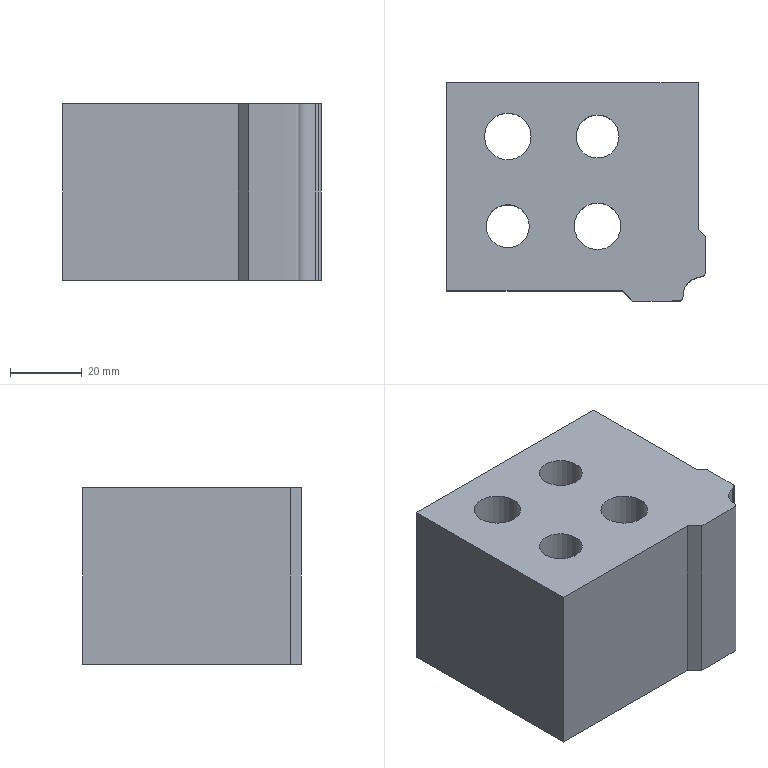Part | NX | features solid 2 | 1 solid | 20 faces | box 72 x 60.859 x 49.284 mm | volume 170289 mm3 | plane 11 | cylinder 7 | spline 2 | commonest cylinder face diameters 12 x2 13 x2 20 x2 2 x1
STEP:
#1=CARTESIAN_POINT('',(-548.,845.,-149.284));
#2=VERTEX_POINT('',#1);
#3=CARTESIAN_POINT('',(-538.,845.,-149.284));
#4=DIRECTION('',(0.,0.,-1.));
#5=DIRECTION('',(-1.,0.,0.));
#6=AXIS2_PLACEMENT_3D('',#3,#4,#5);
#7=CIRCLE('',#6,10.);
#8=EDGE_CURVE('',#2,#2,#7,.T.);
#9=ORIENTED_EDGE('',*,*,#8,.F.);
#10=EDGE_LOOP('',(#9));
#11=FACE_BOUND('',#10,.T.);
#12=CARTESIAN_POINT('',(-544.,820.,-149.284));
#13=VERTEX_POINT('',#12);
#14=CARTESIAN_POINT('',(-538.,820.,-149.284));
#15=DIRECTION('',(0.,0.,-1.));
#16=DIRECTION('',(-1.,0.,0.));
#17=AXIS2_PLACEMENT_3D('',#14,#15,#16);
#18=CIRCLE('',#17,6.);
#19=EDGE_CURVE('',#13,#13,#18,.T.);
#20=ORIENTED_EDGE('',*,*,#19,.F.);
#21=EDGE_LOOP('',(#20));
#22=FACE_BOUND('',#21,.T.);
#23=CARTESIAN_POINT('',(-519.,845.,-149.284));
#24=VERTEX_POINT('',#23);
#25=CARTESIAN_POINT('',(-513.,845.,-149.284));
#26=DIRECTION('',(0.,0.,-1.));
#27=DIRECTION('',(-1.,0.,0.));
#28=AXIS2_PLACEMENT_3D('',#25,#26,#27);
#29=CIRCLE('',#28,6.);
#30=EDGE_CURVE('',#24,#24,#29,.T.);
#31=ORIENTED_EDGE('',*,*,#30,.F.);
#32=EDGE_LOOP('',(#31));
#33=FACE_BOUND('',#32,.T.);
#34=CARTESIAN_POINT('',(-523.,820.,-149.284));
#35=VERTEX_POINT('',#34);
#36=CARTESIAN_POINT('',(-513.,820.,-149.284));
#37=DIRECTION('',(0.,0.,-1.));
#38=DIRECTION('',(-1.,0.,0.));
#39=AXIS2_PLACEMENT_3D('',#36,#37,#38);
#40=CIRCLE('',#39,10.);
#41=EDGE_CURVE('',#35,#35,#40,.T.);
#42=ORIENTED_EDGE('',*,*,#41,.F.);
#43=EDGE_LOOP('',(#42));
#44=FACE_BOUND('',#43,.T.);
#45=CARTESIAN_POINT('',(-503.223,799.156,-149.284));
#46=VERTEX_POINT('',#45);
#47=CARTESIAN_POINT('',(-484.629,805.851,-149.284));
#48=VERTEX_POINT('',#47);
#49=CARTESIAN_POINT('',(-534.002,799.156,-149.284));
#50=CARTESIAN_POINT('',(-520.407,799.156,-149.284));
#51=CARTESIAN_POINT('',(-506.812,799.156,-149.284));
#52=CARTESIAN_POINT('',(-493.216,799.156,-149.284));
#53=CARTESIAN_POINT('',(-492.716,799.156,-149.284));
#54=CARTESIAN_POINT('',(-491.716,799.156,-149.284));
#55=CARTESIAN_POINT('',(-490.649,799.128,-149.284));
#56=CARTESIAN_POINT('',(-490.021,799.17,-149.284));
#57=CARTESIAN_POINT('',(-489.772,799.252,-149.284));
#58=CARTESIAN_POINT('',(-489.501,799.442,-149.284));
#59=CARTESIAN_POINT('',(-489.316,799.721,-149.284));
#60=CARTESIAN_POINT('',(-489.236,799.97,-149.284));
#61=CARTESIAN_POINT('',(-489.184,800.499,-149.284));
#62=CARTESIAN_POINT('',(-489.152,801.357,-149.284));
#63=CARTESIAN_POINT('',(-488.826,802.918,-149.284));
#64=CARTESIAN_POINT('',(-487.668,804.644,-149.284));
#65=CARTESIAN_POINT('',(-485.756,805.629,-149.284));
#66=CARTESIAN_POINT('',(-484.079,805.973,-149.284));
#67=CARTESIAN_POINT('',(-483.087,806.009,-149.284));
#68=CARTESIAN_POINT('',(-482.401,806.124,-149.284));
#69=CARTESIAN_POINT('',(-482.07,806.341,-149.284));
#70=CARTESIAN_POINT('',(-481.846,806.67,-149.284));
#71=CARTESIAN_POINT('',(-481.753,807.261,-149.284));
#72=CARTESIAN_POINT('',(-481.79,808.059,-149.284));
#73=CARTESIAN_POINT('',(-481.79,808.726,-149.284));
#74=CARTESIAN_POINT('',(-481.79,809.059,-149.284));
#75=CARTESIAN_POINT('',(-481.79,822.654,-149.284));
#76=CARTESIAN_POINT('',(-481.79,836.249,-149.284));
#77=CARTESIAN_POINT('',(-481.79,849.844,-149.284));
#78=B_SPLINE_CURVE_WITH_KNOTS('',3,(#49,#50,#51,#52,#53,#54,#55,#56,#57,#58,#59,#60,#61,#62,#63,#64,#65,#66,#67,#68,#69,#70,#71,#72,#73,#74,#75,#76,#77),.UNSPECIFIED.,.F.,.F.,(4,3,1,1,1,1,1,1,1,1,1,1,1,1,1,1,1,1,1,1,1,3,4),(0.,0.4079,0.4228,0.4378,0.4398,0.4418,0.4457,0.4496,0.4516,0.4536,0.4664,0.4793,0.5051,0.5308,0.5437,0.5566,0.5605,0.5644,0.5683,0.5722,0.5822,0.5921,1.),.UNSPECIFIED.);
#79=EDGE_CURVE('',#46,#48,#78,.T.);
#80=ORIENTED_EDGE('',*,*,#79,.F.);
#81=CARTESIAN_POINT('',(-506.067,802.,-149.284));
#82=VERTEX_POINT('',#81);
#83=CARTESIAN_POINT('',(-499.067,795.,-149.284));
#84=DIRECTION('',(-0.7071,0.7071,0.));
#85=VECTOR('',#84,1000.);
#86=LINE('',#83,#85);
#87=EDGE_CURVE('',#82,#46,#86,.F.);
#88=ORIENTED_EDGE('',*,*,#87,.F.);
#89=CARTESIAN_POINT('',(-555.,802.,-149.284));
#90=VERTEX_POINT('',#89);
#91=CARTESIAN_POINT('',(-504.067,802.,-149.284));
#92=DIRECTION('',(-1.,0.,0.));
#93=VECTOR('',#92,1000.);
#94=LINE('',#91,#93);
#95=EDGE_CURVE('',#90,#82,#94,.F.);
#96=ORIENTED_EDGE('',*,*,#95,.F.);
#97=CARTESIAN_POINT('',(-555.,860.,-149.284));
#98=VERTEX_POINT('',#97);
#99=CARTESIAN_POINT('',(-555.,800.,-149.284));
#100=DIRECTION('',(0.,1.,0.));
#101=VECTOR('',#100,1000.);
#102=LINE('',#99,#101);
#103=EDGE_CURVE('',#98,#90,#102,.F.);
#104=ORIENTED_EDGE('',*,*,#103,.F.);
#105=CARTESIAN_POINT('',(-485.,860.,-149.284));
#106=VERTEX_POINT('',#105);
#107=CARTESIAN_POINT('',(-488.,860.,-149.284));
#108=DIRECTION('',(-1.,0.,0.));
#109=VECTOR('',#108,1000.);
#110=LINE('',#107,#109);
#111=EDGE_CURVE('',#98,#106,#110,.F.);
#112=ORIENTED_EDGE('',*,*,#111,.T.);
#113=CARTESIAN_POINT('',(-485.,819.091,-149.284));
#114=VERTEX_POINT('',#113);
#115=CARTESIAN_POINT('',(-485.,822.091,-149.284));
#116=DIRECTION('',(0.,1.,0.));
#117=VECTOR('',#116,1000.);
#118=LINE('',#115,#117);
#119=EDGE_CURVE('',#106,#114,#118,.F.);
#120=ORIENTED_EDGE('',*,*,#119,.T.);
#121=CARTESIAN_POINT('',(-483.,817.091,-149.284));
#122=VERTEX_POINT('',#121);
#123=CARTESIAN_POINT('',(-483.,817.091,-149.284));
#124=DIRECTION('',(-0.7071,0.7071,0.));
#125=VECTOR('',#124,1000.);
#126=LINE('',#123,#125);
#127=EDGE_CURVE('',#114,#122,#126,.F.);
#128=ORIENTED_EDGE('',*,*,#127,.T.);
#129=CARTESIAN_POINT('',(-483.,807.091,-149.284));
#130=VERTEX_POINT('',#129);
#131=CARTESIAN_POINT('',(-483.,807.091,-149.284));
#132=DIRECTION('',(0.,1.,0.));
#133=VECTOR('',#132,1000.);
#134=LINE('',#131,#133);
#135=EDGE_CURVE('',#122,#130,#134,.F.);
#136=ORIENTED_EDGE('',*,*,#135,.T.);
#137=CARTESIAN_POINT('',(-483.777,806.116,-149.284));
#138=VERTEX_POINT('',#137);
#139=CARTESIAN_POINT('',(-484.,807.091,-149.284));
#140=DIRECTION('',(0.,0.,-1.));
#141=DIRECTION('',(-1.,0.,0.));
#142=AXIS2_PLACEMENT_3D('',#139,#140,#141);
#143=CIRCLE('',#142,1.);
#144=EDGE_CURVE('',#130,#138,#143,.T.);
#145=ORIENTED_EDGE('',*,*,#144,.T.);
#146=CARTESIAN_POINT('',(-483.777,806.116,-149.284));
#147=CARTESIAN_POINT('',(-484.07,806.049,-149.284));
#148=CARTESIAN_POINT('',(-484.354,805.962,-149.284));
#149=CARTESIAN_POINT('',(-484.629,805.851,-149.284));
#150=B_SPLINE_CURVE_WITH_KNOTS('',3,(#146,#147,#148,#149),.UNSPECIFIED.,.F.,.F.,(4,4),(0.,0.000889),.UNSPECIFIED.);
#151=EDGE_CURVE('',#138,#48,#150,.T.);
#152=ORIENTED_EDGE('',*,*,#151,.T.);
#153=EDGE_LOOP('',(#80,#88,#96,#104,#112,#120,#128,#136,#145,#152));
#154=FACE_BOUND('',#153,.T.);
#155=CARTESIAN_POINT('',(-594.308,845.,-149.284));
#156=DIRECTION('',(0.,0.,-1.));
#157=DIRECTION('',(-1.,0.,0.));
#158=AXIS2_PLACEMENT_3D('',#155,#156,#157);
#159=PLANE('',#158);
#160=ADVANCED_FACE('',(#11,#22,#33,#44,#154),#159,.T.);
#161=CARTESIAN_POINT('',(-484.629,805.851,-100.));
#162=VERTEX_POINT('',#161);
#163=CARTESIAN_POINT('',(-503.223,799.156,-100.));
#164=VERTEX_POINT('',#163);
#165=CARTESIAN_POINT('',(-534.002,799.156,-100.));
#166=CARTESIAN_POINT('',(-520.407,799.156,-100.));
#167=CARTESIAN_POINT('',(-506.812,799.156,-100.));
#168=CARTESIAN_POINT('',(-493.216,799.156,-100.));
#169=CARTESIAN_POINT('',(-492.716,799.156,-100.));
#170=CARTESIAN_POINT('',(-491.716,799.156,-100.));
#171=CARTESIAN_POINT('',(-490.649,799.128,-100.));
#172=CARTESIAN_POINT('',(-490.021,799.17,-100.));
#173=CARTESIAN_POINT('',(-489.772,799.252,-100.));
#174=CARTESIAN_POINT('',(-489.501,799.442,-100.));
#175=CARTESIAN_POINT('',(-489.316,799.721,-100.));
#176=CARTESIAN_POINT('',(-489.236,799.97,-100.));
#177=CARTESIAN_POINT('',(-489.184,800.499,-100.));
#178=CARTESIAN_POINT('',(-489.152,801.357,-100.));
#179=CARTESIAN_POINT('',(-488.826,802.918,-100.));
#180=CARTESIAN_POINT('',(-487.668,804.644,-100.));
#181=CARTESIAN_POINT('',(-485.756,805.629,-100.));
#182=CARTESIAN_POINT('',(-484.079,805.973,-100.));
#183=CARTESIAN_POINT('',(-483.087,806.009,-100.));
#184=CARTESIAN_POINT('',(-482.401,806.124,-100.));
#185=CARTESIAN_POINT('',(-482.07,806.341,-100.));
#186=CARTESIAN_POINT('',(-481.846,806.67,-100.));
#187=CARTESIAN_POINT('',(-481.753,807.261,-100.));
#188=CARTESIAN_POINT('',(-481.79,808.059,-100.));
#189=CARTESIAN_POINT('',(-481.79,808.726,-100.));
#190=CARTESIAN_POINT('',(-481.79,809.059,-100.));
#191=CARTESIAN_POINT('',(-481.79,822.654,-100.));
#192=CARTESIAN_POINT('',(-481.79,836.249,-100.));
#193=CARTESIAN_POINT('',(-481.79,849.844,-100.));
#194=B_SPLINE_CURVE_WITH_KNOTS('',3,(#165,#166,#167,#168,#169,#170,#171,#172,#173,#174,#175,#176,#177,#178,#179,#180,#181,#182,#183,#184,#185,#186,#187,#188,#189,#190,#191,#192,#193),.UNSPECIFIED.,.F.,.F.,(4,3,1,1,1,1,1,1,1,1,1,1,1,1,1,1,1,1,1,1,1,3,4),(0.,0.4079,0.4228,0.4378,0.4398,0.4418,0.4457,0.4496,0.4516,0.4536,0.4664,0.4793,0.5051,0.5308,0.5437,0.5566,0.5605,0.5644,0.5683,0.5722,0.5822,0.5921,1.),.UNSPECIFIED.);
#195=EDGE_CURVE('',#162,#164,#194,.F.);
#196=ORIENTED_EDGE('',*,*,#195,.F.);
#197=CARTESIAN_POINT('',(-483.777,806.116,-100.));
#198=VERTEX_POINT('',#197);
#199=CARTESIAN_POINT('',(-484.629,805.851,-100.));
#200=CARTESIAN_POINT('',(-484.353,805.962,-100.));
#201=CARTESIAN_POINT('',(-484.069,806.049,-100.));
#202=CARTESIAN_POINT('',(-483.777,806.116,-100.));
#203=B_SPLINE_CURVE_WITH_KNOTS('',3,(#199,#200,#201,#202),.UNSPECIFIED.,.F.,.F.,(4,4),(0.06032,0.06122),.UNSPECIFIED.);
#204=EDGE_CURVE('',#162,#198,#203,.T.);
#205=ORIENTED_EDGE('',*,*,#204,.T.);
#206=CARTESIAN_POINT('',(-483.,807.091,-100.));
#207=VERTEX_POINT('',#206);
#208=CARTESIAN_POINT('',(-484.,807.091,-100.));
#209=DIRECTION('',(0.,0.,1.));
#210=DIRECTION('',(1.,0.,0.));
#211=AXIS2_PLACEMENT_3D('',#208,#209,#210);
#212=CIRCLE('',#211,1.);
#213=EDGE_CURVE('',#198,#207,#212,.T.);
#214=ORIENTED_EDGE('',*,*,#213,.T.);
#215=CARTESIAN_POINT('',(-483.,817.091,-100.));
#216=VERTEX_POINT('',#215);
#217=CARTESIAN_POINT('',(-483.,808.547,-100.));
#218=DIRECTION('',(0.,1.,0.));
#219=VECTOR('',#218,1000.);
#220=LINE('',#217,#219);
#221=EDGE_CURVE('',#207,#216,#220,.T.);
#222=ORIENTED_EDGE('',*,*,#221,.T.);
#223=CARTESIAN_POINT('',(-485.,819.091,-100.));
#224=VERTEX_POINT('',#223);
#225=CARTESIAN_POINT('',(-485.119,819.209,-100.));
#226=DIRECTION('',(-0.7071,0.7071,0.));
#227=VECTOR('',#226,1000.);
#228=LINE('',#225,#227);
#229=EDGE_CURVE('',#216,#224,#228,.T.);
#230=ORIENTED_EDGE('',*,*,#229,.T.);
#231=CARTESIAN_POINT('',(-485.,860.,-100.));
#232=VERTEX_POINT('',#231);
#233=CARTESIAN_POINT('',(-485.,808.547,-100.));
#234=DIRECTION('',(0.,1.,0.));
#235=VECTOR('',#234,1000.);
#236=LINE('',#233,#235);
#237=EDGE_CURVE('',#224,#232,#236,.T.);
#238=ORIENTED_EDGE('',*,*,#237,.T.);
#239=CARTESIAN_POINT('',(-555.,860.,-100.));
#240=VERTEX_POINT('',#239);
#241=CARTESIAN_POINT('',(-495.781,860.,-100.));
#242=DIRECTION('',(-1.,0.,0.));
#243=VECTOR('',#242,1000.);
#244=LINE('',#241,#243);
#245=EDGE_CURVE('',#232,#240,#244,.T.);
#246=ORIENTED_EDGE('',*,*,#245,.T.);
#247=CARTESIAN_POINT('',(-555.,802.,-100.));
#248=VERTEX_POINT('',#247);
#249=CARTESIAN_POINT('',(-555.,808.547,-100.));
#250=DIRECTION('',(0.,1.,0.));
#251=VECTOR('',#250,1000.);
#252=LINE('',#249,#251);
#253=EDGE_CURVE('',#248,#240,#252,.T.);
#254=ORIENTED_EDGE('',*,*,#253,.F.);
#255=CARTESIAN_POINT('',(-506.067,802.,-100.));
#256=VERTEX_POINT('',#255);
#257=CARTESIAN_POINT('',(-495.781,802.,-100.));
#258=DIRECTION('',(-1.,0.,0.));
#259=VECTOR('',#258,1000.);
#260=LINE('',#257,#259);
#261=EDGE_CURVE('',#256,#248,#260,.T.);
#262=ORIENTED_EDGE('',*,*,#261,.F.);
#263=CARTESIAN_POINT('',(-504.197,800.131,-100.));
#264=DIRECTION('',(-0.7071,0.7071,0.));
#265=VECTOR('',#264,1000.);
#266=LINE('',#263,#265);
#267=EDGE_CURVE('',#164,#256,#266,.T.);
#268=ORIENTED_EDGE('',*,*,#267,.F.);
#269=EDGE_LOOP('',(#196,#205,#214,#222,#230,#238,#246,#254,#262,#268));
#270=FACE_BOUND('',#269,.T.);
#271=CARTESIAN_POINT('',(-506.5,820.,-100.));
#272=VERTEX_POINT('',#271);
#273=CARTESIAN_POINT('',(-513.,820.,-100.));
#274=DIRECTION('',(0.,0.,1.));
#275=DIRECTION('',(1.,0.,0.));
#276=AXIS2_PLACEMENT_3D('',#273,#274,#275);
#277=CIRCLE('',#276,6.5);
#278=EDGE_CURVE('',#272,#272,#277,.T.);
#279=ORIENTED_EDGE('',*,*,#278,.F.);
#280=EDGE_LOOP('',(#279));
#281=FACE_BOUND('',#280,.T.);
#282=CARTESIAN_POINT('',(-531.5,845.,-100.));
#283=VERTEX_POINT('',#282);
#284=CARTESIAN_POINT('',(-538.,845.,-100.));
#285=DIRECTION('',(0.,0.,1.));
#286=DIRECTION('',(1.,0.,0.));
#287=AXIS2_PLACEMENT_3D('',#284,#285,#286);
#288=CIRCLE('',#287,6.5);
#289=EDGE_CURVE('',#283,#283,#288,.T.);
#290=ORIENTED_EDGE('',*,*,#289,.F.);
#291=EDGE_LOOP('',(#290));
#292=FACE_BOUND('',#291,.T.);
#293=CARTESIAN_POINT('',(-507.,845.,-100.));
#294=VERTEX_POINT('',#293);
#295=CARTESIAN_POINT('',(-513.,845.,-100.));
#296=DIRECTION('',(0.,0.,1.));
#297=DIRECTION('',(1.,0.,0.));
#298=AXIS2_PLACEMENT_3D('',#295,#296,#297);
#299=CIRCLE('',#298,6.);
#300=EDGE_CURVE('',#294,#294,#299,.F.);
#301=ORIENTED_EDGE('',*,*,#300,.T.);
#302=EDGE_LOOP('',(#301));
#303=FACE_BOUND('',#302,.T.);
#304=CARTESIAN_POINT('',(-532.,820.,-100.));
#305=VERTEX_POINT('',#304);
#306=CARTESIAN_POINT('',(-538.,820.,-100.));
#307=DIRECTION('',(0.,0.,1.));
#308=DIRECTION('',(1.,0.,0.));
#309=AXIS2_PLACEMENT_3D('',#306,#307,#308);
#310=CIRCLE('',#309,6.);
#311=EDGE_CURVE('',#305,#305,#310,.F.);
#312=ORIENTED_EDGE('',*,*,#311,.T.);
#313=EDGE_LOOP('',(#312));
#314=FACE_BOUND('',#313,.T.);
#315=CARTESIAN_POINT('',(-495.781,808.547,-100.));
#316=DIRECTION('',(0.,0.,1.));
#317=DIRECTION('',(1.,0.,0.));
#318=AXIS2_PLACEMENT_3D('',#315,#316,#317);
#319=PLANE('',#318);
#320=ADVANCED_FACE('',(#270,#281,#292,#303,#314),#319,.T.);
#321=CARTESIAN_POINT('',(-555.,860.,-505.));
#322=DIRECTION('',(0.,0.,1.));
#323=VECTOR('',#322,1000.);
#324=LINE('',#321,#323);
#325=EDGE_CURVE('',#98,#240,#324,.T.);
#326=ORIENTED_EDGE('',*,*,#325,.F.);
#327=ORIENTED_EDGE('',*,*,#103,.T.);
#328=CARTESIAN_POINT('',(-555.,802.,-505.));
#329=DIRECTION('',(0.,0.,1.));
#330=VECTOR('',#329,1000.);
#331=LINE('',#328,#330);
#332=EDGE_CURVE('',#90,#248,#331,.T.);
#333=ORIENTED_EDGE('',*,*,#332,.T.);
#334=ORIENTED_EDGE('',*,*,#253,.T.);
#335=EDGE_LOOP('',(#326,#327,#333,#334));
#336=FACE_BOUND('',#335,.T.);
#337=CARTESIAN_POINT('',(-555.,800.,-505.));
#338=DIRECTION('',(1.,0.,0.));
#339=DIRECTION('',(0.,0.,-1.));
#340=AXIS2_PLACEMENT_3D('',#337,#338,#339);
#341=PLANE('',#340);
#342=ADVANCED_FACE('',(#336),#341,.F.);
#343=ORIENTED_EDGE('',*,*,#332,.F.);
#344=ORIENTED_EDGE('',*,*,#95,.T.);
#345=CARTESIAN_POINT('',(-506.067,802.,-505.));
#346=DIRECTION('',(0.,0.,1.));
#347=VECTOR('',#346,1000.);
#348=LINE('',#345,#347);
#349=EDGE_CURVE('',#82,#256,#348,.T.);
#350=ORIENTED_EDGE('',*,*,#349,.T.);
#351=ORIENTED_EDGE('',*,*,#261,.T.);
#352=EDGE_LOOP('',(#343,#344,#350,#351));
#353=FACE_BOUND('',#352,.T.);
#354=CARTESIAN_POINT('',(-504.067,802.,-505.));
#355=DIRECTION('',(0.,1.,0.));
#356=DIRECTION('',(0.,0.,1.));
#357=AXIS2_PLACEMENT_3D('',#354,#355,#356);
#358=PLANE('',#357);
#359=ADVANCED_FACE('',(#353),#358,.F.);
#360=ORIENTED_EDGE('',*,*,#87,.T.);
#361=CARTESIAN_POINT('',(-503.223,799.156,495.));
#362=DIRECTION('',(0.,0.,-1.));
#363=VECTOR('',#362,1000.);
#364=LINE('',#361,#363);
#365=EDGE_CURVE('',#46,#164,#364,.F.);
#366=ORIENTED_EDGE('',*,*,#365,.T.);
#367=ORIENTED_EDGE('',*,*,#267,.T.);
#368=ORIENTED_EDGE('',*,*,#349,.F.);
#369=EDGE_LOOP('',(#360,#366,#367,#368));
#370=FACE_BOUND('',#369,.T.);
#371=CARTESIAN_POINT('',(-499.067,795.,-505.));
#372=DIRECTION('',(0.7071,0.7071,0.));
#373=DIRECTION('',(-0.7071,0.7071,0.));
#374=AXIS2_PLACEMENT_3D('',#371,#372,#373);
#375=PLANE('',#374);
#376=ADVANCED_FACE('',(#370),#375,.F.);
#377=CARTESIAN_POINT('',(-484.629,805.851,495.));
#378=DIRECTION('',(0.,0.,-1.));
#379=VECTOR('',#378,1000.);
#380=LINE('',#377,#379);
#381=EDGE_CURVE('',#48,#162,#380,.F.);
#382=ORIENTED_EDGE('',*,*,#381,.F.);
#383=ORIENTED_EDGE('',*,*,#151,.F.);
#384=CARTESIAN_POINT('',(-483.777,806.116,-505.));
#385=DIRECTION('',(0.,0.,1.));
#386=VECTOR('',#385,1000.);
#387=LINE('',#384,#386);
#388=EDGE_CURVE('',#138,#198,#387,.T.);
#389=ORIENTED_EDGE('',*,*,#388,.T.);
#390=ORIENTED_EDGE('',*,*,#204,.F.);
#391=EDGE_LOOP('',(#382,#383,#389,#390));
#392=FACE_BOUND('',#391,.T.);
#393=CARTESIAN_POINT('',(-484.629,805.851,-149.284));
#394=CARTESIAN_POINT('',(-484.629,805.851,-100.));
#395=CARTESIAN_POINT('',(-484.354,805.962,-149.284));
#396=CARTESIAN_POINT('',(-484.354,805.962,-100.));
#397=CARTESIAN_POINT('',(-484.069,806.049,-149.284));
#398=CARTESIAN_POINT('',(-484.069,806.049,-100.));
#399=CARTESIAN_POINT('',(-483.777,806.116,-149.284));
#400=CARTESIAN_POINT('',(-483.777,806.116,-100.));
#401=B_SPLINE_SURFACE_WITH_KNOTS('',3,1,((#393,#394),(#395,#396),(#397,#398),(#399,#400)),.SURF_OF_LINEAR_EXTRUSION.,.F.,.F.,.F.,(4,4),(2,2),(0.9197,0.987),(0.,1.),.PIECEWISE_BEZIER_KNOTS.);
#402=ADVANCED_FACE('',(#392),#401,.T.);
#403=ORIENTED_EDGE('',*,*,#144,.F.);
#404=CARTESIAN_POINT('',(-483.,807.091,-505.));
#405=DIRECTION('',(0.,0.,1.));
#406=VECTOR('',#405,1000.);
#407=LINE('',#404,#406);
#408=EDGE_CURVE('',#130,#207,#407,.T.);
#409=ORIENTED_EDGE('',*,*,#408,.T.);
#410=ORIENTED_EDGE('',*,*,#213,.F.);
#411=ORIENTED_EDGE('',*,*,#388,.F.);
#412=EDGE_LOOP('',(#403,#409,#410,#411));
#413=FACE_BOUND('',#412,.T.);
#414=CARTESIAN_POINT('',(-484.,807.091,-505.));
#415=DIRECTION('',(0.,0.,1.));
#416=DIRECTION('',(1.,0.,0.));
#417=AXIS2_PLACEMENT_3D('',#414,#415,#416);
#418=CYLINDRICAL_SURFACE('',#417,1.);
#419=ADVANCED_FACE('',(#413),#418,.T.);
#420=ORIENTED_EDGE('',*,*,#135,.F.);
#421=CARTESIAN_POINT('',(-483.,817.091,-505.));
#422=DIRECTION('',(0.,0.,1.));
#423=VECTOR('',#422,1000.);
#424=LINE('',#421,#423);
#425=EDGE_CURVE('',#122,#216,#424,.T.);
#426=ORIENTED_EDGE('',*,*,#425,.T.);
#427=ORIENTED_EDGE('',*,*,#221,.F.);
#428=ORIENTED_EDGE('',*,*,#408,.F.);
#429=EDGE_LOOP('',(#420,#426,#427,#428));
#430=FACE_BOUND('',#429,.T.);
#431=CARTESIAN_POINT('',(-483.,807.091,-505.));
#432=DIRECTION('',(1.,0.,0.));
#433=DIRECTION('',(0.,0.,-1.));
#434=AXIS2_PLACEMENT_3D('',#431,#432,#433);
#435=PLANE('',#434);
#436=ADVANCED_FACE('',(#430),#435,.T.);
#437=ORIENTED_EDGE('',*,*,#127,.F.);
#438=CARTESIAN_POINT('',(-485.,819.091,-505.));
#439=DIRECTION('',(0.,0.,1.));
#440=VECTOR('',#439,1000.);
#441=LINE('',#438,#440);
#442=EDGE_CURVE('',#114,#224,#441,.T.);
#443=ORIENTED_EDGE('',*,*,#442,.T.);
#444=ORIENTED_EDGE('',*,*,#229,.F.);
#445=ORIENTED_EDGE('',*,*,#425,.F.);
#446=EDGE_LOOP('',(#437,#443,#444,#445));
#447=FACE_BOUND('',#446,.T.);
#448=CARTESIAN_POINT('',(-483.,817.091,-505.));
#449=DIRECTION('',(0.7071,0.7071,0.));
#450=DIRECTION('',(-0.7071,0.7071,0.));
#451=AXIS2_PLACEMENT_3D('',#448,#449,#450);
#452=PLANE('',#451);
#453=ADVANCED_FACE('',(#447),#452,.T.);
#454=ORIENTED_EDGE('',*,*,#119,.F.);
#455=CARTESIAN_POINT('',(-485.,860.,-505.));
#456=DIRECTION('',(0.,0.,1.));
#457=VECTOR('',#456,1000.);
#458=LINE('',#455,#457);
#459=EDGE_CURVE('',#106,#232,#458,.T.);
#460=ORIENTED_EDGE('',*,*,#459,.T.);
#461=ORIENTED_EDGE('',*,*,#237,.F.);
#462=ORIENTED_EDGE('',*,*,#442,.F.);
#463=EDGE_LOOP('',(#454,#460,#461,#462));
#464=FACE_BOUND('',#463,.T.);
#465=CARTESIAN_POINT('',(-485.,822.091,-505.));
#466=DIRECTION('',(1.,0.,0.));
#467=DIRECTION('',(0.,0.,-1.));
#468=AXIS2_PLACEMENT_3D('',#465,#466,#467);
#469=PLANE('',#468);
#470=ADVANCED_FACE('',(#464),#469,.T.);
#471=ORIENTED_EDGE('',*,*,#111,.F.);
#472=ORIENTED_EDGE('',*,*,#325,.T.);
#473=ORIENTED_EDGE('',*,*,#245,.F.);
#474=ORIENTED_EDGE('',*,*,#459,.F.);
#475=EDGE_LOOP('',(#471,#472,#473,#474));
#476=FACE_BOUND('',#475,.T.);
#477=CARTESIAN_POINT('',(-488.,860.,-505.));
#478=DIRECTION('',(0.,1.,0.));
#479=DIRECTION('',(0.,0.,1.));
#480=AXIS2_PLACEMENT_3D('',#477,#478,#479);
#481=PLANE('',#480);
#482=ADVANCED_FACE('',(#476),#481,.T.);
#483=ORIENTED_EDGE('',*,*,#300,.F.);
#484=EDGE_LOOP('',(#483));
#485=FACE_BOUND('',#484,.T.);
#486=ORIENTED_EDGE('',*,*,#30,.T.);
#487=EDGE_LOOP('',(#486));
#488=FACE_BOUND('',#487,.T.);
#489=CARTESIAN_POINT('',(-513.,845.,-5.));
#490=DIRECTION('',(0.,0.,-1.));
#491=DIRECTION('',(-1.,0.,0.));
#492=AXIS2_PLACEMENT_3D('',#489,#490,#491);
#493=CYLINDRICAL_SURFACE('',#492,6.);
#494=ADVANCED_FACE('',(#485,#488),#493,.F.);
#495=ORIENTED_EDGE('',*,*,#311,.F.);
#496=EDGE_LOOP('',(#495));
#497=FACE_BOUND('',#496,.T.);
#498=ORIENTED_EDGE('',*,*,#19,.T.);
#499=EDGE_LOOP('',(#498));
#500=FACE_BOUND('',#499,.T.);
#501=CARTESIAN_POINT('',(-538.,820.,-5.));
#502=DIRECTION('',(0.,0.,-1.));
#503=DIRECTION('',(-1.,0.,0.));
#504=AXIS2_PLACEMENT_3D('',#501,#502,#503);
#505=CYLINDRICAL_SURFACE('',#504,6.);
#506=ADVANCED_FACE('',(#497,#500),#505,.F.);
#507=CARTESIAN_POINT('',(-531.5,845.,-125.));
#508=VERTEX_POINT('',#507);
#509=CARTESIAN_POINT('',(-538.,845.,-125.));
#510=DIRECTION('',(0.,0.,1.));
#511=DIRECTION('',(1.,0.,0.));
#512=AXIS2_PLACEMENT_3D('',#509,#510,#511);
#513=CIRCLE('',#512,6.5);
#514=EDGE_CURVE('',#508,#508,#513,.F.);
#515=ORIENTED_EDGE('',*,*,#514,.T.);
#516=EDGE_LOOP('',(#515));
#517=FACE_BOUND('',#516,.T.);
#518=ORIENTED_EDGE('',*,*,#289,.T.);
#519=EDGE_LOOP('',(#518));
#520=FACE_BOUND('',#519,.T.);
#521=CARTESIAN_POINT('',(-538.,845.,-125.));
#522=DIRECTION('',(0.,0.,1.));
#523=DIRECTION('',(1.,0.,0.));
#524=AXIS2_PLACEMENT_3D('',#521,#522,#523);
#525=CYLINDRICAL_SURFACE('',#524,6.5);
#526=ADVANCED_FACE('',(#517,#520),#525,.F.);
#527=CARTESIAN_POINT('',(-506.5,820.,-125.));
#528=VERTEX_POINT('',#527);
#529=CARTESIAN_POINT('',(-513.,820.,-125.));
#530=DIRECTION('',(0.,0.,1.));
#531=DIRECTION('',(1.,0.,0.));
#532=AXIS2_PLACEMENT_3D('',#529,#530,#531);
#533=CIRCLE('',#532,6.5);
#534=EDGE_CURVE('',#528,#528,#533,.F.);
#535=ORIENTED_EDGE('',*,*,#534,.T.);
#536=EDGE_LOOP('',(#535));
#537=FACE_BOUND('',#536,.T.);
#538=ORIENTED_EDGE('',*,*,#278,.T.);
#539=EDGE_LOOP('',(#538));
#540=FACE_BOUND('',#539,.T.);
#541=CARTESIAN_POINT('',(-513.,820.,-125.));
#542=DIRECTION('',(0.,0.,1.));
#543=DIRECTION('',(1.,0.,0.));
#544=AXIS2_PLACEMENT_3D('',#541,#542,#543);
#545=CYLINDRICAL_SURFACE('',#544,6.5);
#546=ADVANCED_FACE('',(#537,#540),#545,.F.);
#547=CARTESIAN_POINT('',(-503.,820.,-125.));
#548=VERTEX_POINT('',#547);
#549=CARTESIAN_POINT('',(-513.,820.,-125.));
#550=DIRECTION('',(0.,0.,1.));
#551=DIRECTION('',(1.,0.,0.));
#552=AXIS2_PLACEMENT_3D('',#549,#550,#551);
#553=CIRCLE('',#552,10.);
#554=EDGE_CURVE('',#548,#548,#553,.T.);
#555=ORIENTED_EDGE('',*,*,#554,.T.);
#556=EDGE_LOOP('',(#555));
#557=FACE_BOUND('',#556,.T.);
#558=ORIENTED_EDGE('',*,*,#41,.T.);
#559=EDGE_LOOP('',(#558));
#560=FACE_BOUND('',#559,.T.);
#561=CARTESIAN_POINT('',(-513.,820.,-125.));
#562=DIRECTION('',(0.,0.,-1.));
#563=DIRECTION('',(-1.,0.,0.));
#564=AXIS2_PLACEMENT_3D('',#561,#562,#563);
#565=CYLINDRICAL_SURFACE('',#564,10.);
#566=ADVANCED_FACE('',(#557,#560),#565,.F.);
#567=ORIENTED_EDGE('',*,*,#554,.F.);
#568=EDGE_LOOP('',(#567));
#569=FACE_BOUND('',#568,.T.);
#570=ORIENTED_EDGE('',*,*,#534,.F.);
#571=EDGE_LOOP('',(#570));
#572=FACE_BOUND('',#571,.T.);
#573=CARTESIAN_POINT('',(-513.,820.,-125.));
#574=DIRECTION('',(0.,0.,1.));
#575=DIRECTION('',(1.,0.,0.));
#576=AXIS2_PLACEMENT_3D('',#573,#574,#575);
#577=PLANE('',#576);
#578=ADVANCED_FACE('',(#569,#572),#577,.F.);
#579=CARTESIAN_POINT('',(-528.,845.,-125.));
#580=VERTEX_POINT('',#579);
#581=CARTESIAN_POINT('',(-538.,845.,-125.));
#582=DIRECTION('',(0.,0.,1.));
#583=DIRECTION('',(1.,0.,0.));
#584=AXIS2_PLACEMENT_3D('',#581,#582,#583);
#585=CIRCLE('',#584,10.);
#586=EDGE_CURVE('',#580,#580,#585,.T.);
#587=ORIENTED_EDGE('',*,*,#586,.T.);
#588=EDGE_LOOP('',(#587));
#589=FACE_BOUND('',#588,.T.);
#590=ORIENTED_EDGE('',*,*,#8,.T.);
#591=EDGE_LOOP('',(#590));
#592=FACE_BOUND('',#591,.T.);
#593=CARTESIAN_POINT('',(-538.,845.,-125.));
#594=DIRECTION('',(0.,0.,-1.));
#595=DIRECTION('',(-1.,0.,0.));
#596=AXIS2_PLACEMENT_3D('',#593,#594,#595);
#597=CYLINDRICAL_SURFACE('',#596,10.);
#598=ADVANCED_FACE('',(#589,#592),#597,.F.);
#599=ORIENTED_EDGE('',*,*,#586,.F.);
#600=EDGE_LOOP('',(#599));
#601=FACE_BOUND('',#600,.T.);
#602=ORIENTED_EDGE('',*,*,#514,.F.);
#603=EDGE_LOOP('',(#602));
#604=FACE_BOUND('',#603,.T.);
#605=CARTESIAN_POINT('',(-538.,845.,-125.));
#606=DIRECTION('',(0.,0.,1.));
#607=DIRECTION('',(1.,0.,0.));
#608=AXIS2_PLACEMENT_3D('',#605,#606,#607);
#609=PLANE('',#608);
#610=ADVANCED_FACE('',(#601,#604),#609,.F.);
#611=ORIENTED_EDGE('',*,*,#365,.F.);
#612=ORIENTED_EDGE('',*,*,#79,.T.);
#613=ORIENTED_EDGE('',*,*,#381,.T.);
#614=ORIENTED_EDGE('',*,*,#195,.T.);
#615=EDGE_LOOP('',(#611,#612,#613,#614));
#616=FACE_BOUND('',#615,.T.);
#617=CARTESIAN_POINT('',(-503.223,799.156,-100.));
#618=CARTESIAN_POINT('',(-503.223,799.156,-149.284));
#619=CARTESIAN_POINT('',(-502.263,799.156,-100.));
#620=CARTESIAN_POINT('',(-502.263,799.156,-149.284));
#621=CARTESIAN_POINT('',(-500.345,799.156,-100.));
#622=CARTESIAN_POINT('',(-500.345,799.156,-149.284));
#623=CARTESIAN_POINT('',(-497.467,799.156,-100.));
#624=CARTESIAN_POINT('',(-497.467,799.156,-149.284));
#625=CARTESIAN_POINT('',(-495.068,799.155,-100.));
#626=CARTESIAN_POINT('',(-495.068,799.155,-149.284));
#627=CARTESIAN_POINT('',(-493.15,799.157,-100.));
#628=CARTESIAN_POINT('',(-493.15,799.157,-149.284));
#629=CARTESIAN_POINT('',(-491.95,799.152,-100.));
#630=CARTESIAN_POINT('',(-491.95,799.152,-149.284));
#631=CARTESIAN_POINT('',(-490.988,799.143,-100.));
#632=CARTESIAN_POINT('',(-490.988,799.143,-149.284));
#633=CARTESIAN_POINT('',(-490.27,799.124,-100.));
#634=CARTESIAN_POINT('',(-490.27,799.124,-149.284));
#635=CARTESIAN_POINT('',(-489.548,799.292,-100.));
#636=CARTESIAN_POINT('',(-489.548,799.292,-149.284));
#637=CARTESIAN_POINT('',(-489.176,799.981,-100.));
#638=CARTESIAN_POINT('',(-489.176,799.981,-149.284));
#639=CARTESIAN_POINT('',(-489.193,800.655,-100.));
#640=CARTESIAN_POINT('',(-489.193,800.655,-149.284));
#641=CARTESIAN_POINT('',(-489.11,801.544,-100.));
#642=CARTESIAN_POINT('',(-489.11,801.544,-149.284));
#643=CARTESIAN_POINT('',(-488.886,802.634,-100.));
#644=CARTESIAN_POINT('',(-488.886,802.634,-149.284));
#645=CARTESIAN_POINT('',(-488.226,803.824,-100.));
#646=CARTESIAN_POINT('',(-488.226,803.824,-149.284));
#647=CARTESIAN_POINT('',(-486.922,805.121,-100.));
#648=CARTESIAN_POINT('',(-486.922,805.121,-149.284));
#649=CARTESIAN_POINT('',(-485.565,805.667,-100.));
#650=CARTESIAN_POINT('',(-485.565,805.667,-149.284));
#651=CARTESIAN_POINT('',(-484.629,805.851,-100.));
#652=CARTESIAN_POINT('',(-484.629,805.851,-149.284));
#653=B_SPLINE_SURFACE_WITH_KNOTS('',3,1,((#617,#618),(#619,#620),(#621,#622),(#623,#624),(#625,#626),(#627,#628),(#629,#630),(#631,#632),(#633,#634),(#635,#636),(#637,#638),(#639,#640),(#641,#642),(#643,#644),(#645,#646),(#647,#648),(#649,#650),(#651,#652)),.SURF_OF_LINEAR_EXTRUSION.,.F.,.F.,.F.,(4,1,1,1,1,1,1,1,1,1,1,1,1,1,1,4),(2,2),(0.3078,0.3366,0.3654,0.3941,0.4085,0.4229,0.4301,0.4373,0.4445,0.4517,0.4589,0.4661,0.4805,0.4949,0.5093,0.538),(0.,1.),.UNSPECIFIED.);
#654=ADVANCED_FACE('',(#616),#653,.F.);
#655=CLOSED_SHELL('',(#160,#320,#342,#359,#376,#402,#419,#436,#453,#470,#482,#494,#506,#526,#546,#566,#578,#598,#610,#654));
#656=MANIFOLD_SOLID_BREP('',#655);
#657=(LENGTH_UNIT()NAMED_UNIT(*)SI_UNIT(.MILLI.,.METRE.));
#658=UNCERTAINTY_MEASURE_WITH_UNIT(LENGTH_MEASURE(0.0508),#657,'','');
#659=(NAMED_UNIT(*)PLANE_ANGLE_UNIT()SI_UNIT($,.RADIAN.));
#660=(NAMED_UNIT(*)SI_UNIT($,.STERADIAN.)SOLID_ANGLE_UNIT());
#661=(GEOMETRIC_REPRESENTATION_CONTEXT(3)GLOBAL_UNCERTAINTY_ASSIGNED_CONTEXT((#658))GLOBAL_UNIT_ASSIGNED_CONTEXT((#657,#659,#660))REPRESENTATION_CONTEXT('',''));
#662=ADVANCED_BREP_SHAPE_REPRESENTATION('',(#656),#661);